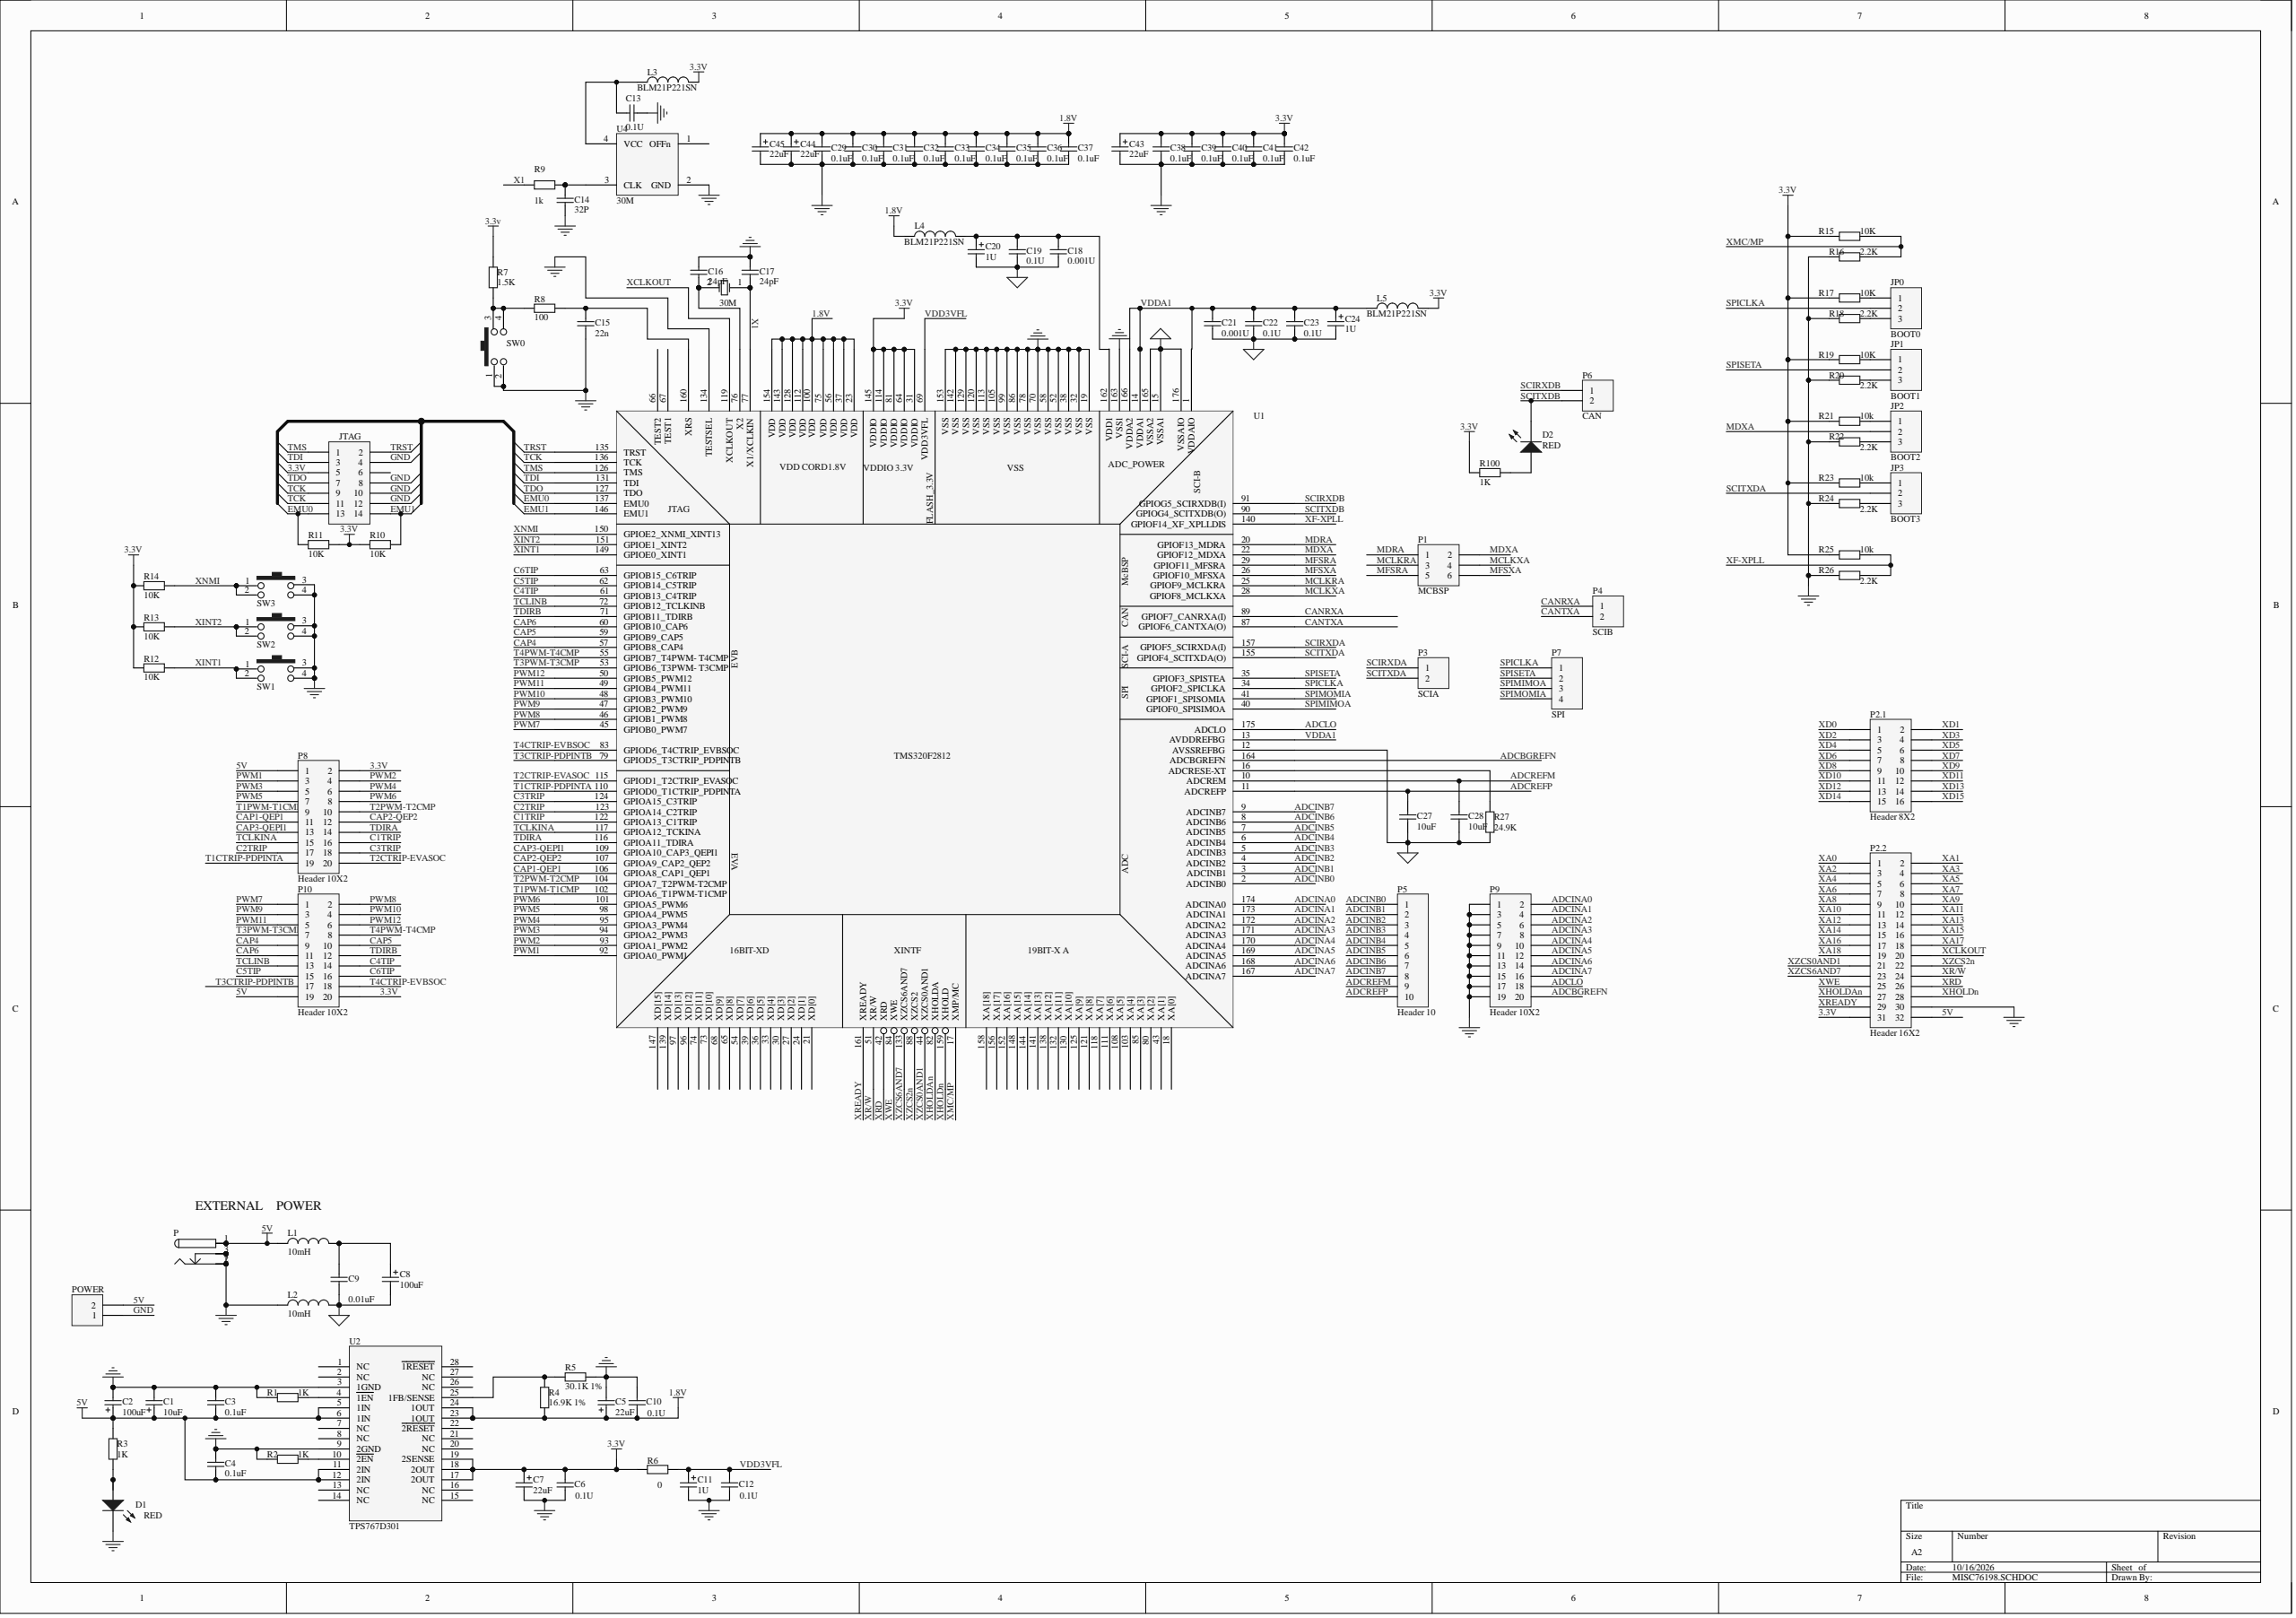Circuit board | Altium Designer | 104 parts | 123 nets
Bill of materials:
Comment,Description,Designator,Footprint,LibRef,Quantity
"XTAL","Crystal Oscillator","30M","TXAL","XTAL","1"
"Cap Pol1","Polarized Capacitor (Radial)","C1, C5, C7","C2","Cap Pol1","3"
"Cap Pol1","Polarized Capacitor (Radial)","C2, C8","C1","Cap Pol1","2"
"Cap","Capacitor","C3, C4, C6, C9, C10, C12, C13, C14, C15, C27, C28","0603","Cap","11"
"Cap Pol1","Polarized Capacitor (Radial)","C11","1210","Cap Pol1","1"
"Cap Semi","Capacitor (Semiconductor SIM Model)","C16, C17, C18, C19, C21, C22, C23","0603","Cap Semi","7"
"Cap Pol1","Polarized Capacitor (Radial)","C20, C24","0805","Cap Pol1","2"
"0.1uF","Capacitor","C29, C30, C31, C32, C33, C34, C35, C36, C37, C38, C39, C40, C41, C42","0603","Cap","14"
"Cap Pol1","Polarized Capacitor (Radial)","C43, C44, C45","1206","Cap Pol1","3"
"RED","Subminiature High Performance AlInGaP LED Lamp","D1, D2","0603","HLMA-PG00-N0011","2"
"BOOT0","Header, 3-Pin","JP0","HDR1X3","Header 3","1"
"BOOT1","Header, 3-Pin","JP1","HDR1X3","Header 3","1"
"BOOT2","Header, 3-Pin","JP2","HDR1X3","Header 3","1"
"BOOT3","Header, 3-Pin","JP3","HDR1X3","Header 3","1"
"Header 7X2","Header, 7-Pin, Dual row","JTAG","HDR2X7","Header 7X2","1"
"Inductor","Inductor","L1, L2, L3, L4, L5","0805","Inductor","5"
"PWR2.5","Low Voltage Power Supply Connector","P","KLD-0202","PWR2.5","1"
"MCBSP","Header, 3-Pin, Dual row","P1","HDR2X3","Header 3X2","1"
"Header 8X2","Header, 8-Pin, Dual row","P2.1","HDR2X8","Header 8X2","1"
"Header 16X2","Header, 16-Pin, Dual row","P2.2","HDR2X16","Header 16X2","1"
"SCIA","Header, 2-Pin","P3","HDR1X2","Header 2","1"
"SCIB","Header, 2-Pin","P4","HDR1X2","Header 2","1"
"Header 10","Header, 10-Pin","P5","HDR1X10","Header 10","1"
"CAN","Header, 2-Pin","P6","HDR1X2","Header 2","1"
"SPI","Header, 4-Pin","P7","HDR1X4","Header 4","1"
"Header 10X2","Header, 10-Pin, Dual row","P8, P9, P10","HDR2X10","Header 10X2","3"
"Header 2","Header, 2-Pin","POWER","HDR1X2","Header 2","1"
"Res2","Resistor","R1, R2, R3, R4, R5, R6, R10, R11, R12, R13, R14, R100","0603","Res2","12"
"1.5K","Resistor","R7","0603","Res2","1"
"100","Resistor","R8","0603","Res2","1"
"1k","Resistor","R9, R16","0603","Res2","2"
"10K","Resistor","R15, R17, R19, R21, R23, R25","0603","Res2","6"
"2.2K","Resistor","R18, R20, R22, R24, R26","0603","Res2","5"
"24.9K","Resistor","R27","0603","Res2","1"
"KEY4","","SW0, SW1, SW2, SW3","key","KEY4","4"
"TMS320F2812","","U1","QFP176","TMS320F2812","1"
"TPS767D301","","U2","TSOP28(0.65mm)","TPS73HD301","1"
"30M","","U4","CRYSTAL1","30M","1"
Netlist (Protel format):
[
30M
TXAL
XTAL



]
[
C1
C2
Cap Pol1



]
[
C2
C1
Cap Pol1



]
[
C3
0603
Cap



]
[
C4
0603
Cap



]
[
C5
C2
Cap Pol1



]
[
C6
0603
Cap



]
[
C7
c2
Cap Pol1



]
[
C8
C1
Cap Pol1



]
[
C9
0603
Cap



]
[
C10
0603
Cap



]
[
C11
1210
Cap Pol1



]
[
C12
0603
Cap



]
[
C13
0603
Cap



]
[
C14
0603
Cap



]
[
C15
0603
Cap



]
[
C16
0603
Cap Semi



]
[
C17
0603
Cap Semi



]
[
C18
0603
Cap Semi



]
[
C19
0603
Cap Semi



]
[
C20
0805
Cap Pol1



]
[
C21
0603
Cap Semi



]
[
C22
0603
Cap Semi



]
[
C23
0603
Cap Semi



]
[
C24
0805
Cap Pol1



]
[
C27
0603
Cap



]
[
C28
0603
Cap



]
[
C29
0603
0.1uF



]
[
C30
0603
0.1uF



]
[
C31
0603
0.1uF



]
[
C32
0603
0.1uF



]
[
C33
0603
0.1uF



]
[
C34
0603
0.1uF



]
[
C35
0603
0.1uF



]
[
C36
0603
0.1uF



]
[
C37
0603
0.1uF



]
[
C38
0603
0.1uF



]
[
C39
0603
0.1uF



]
[
C40
0603
0.1uF



]
[
C41
0603
0.1uF



]
[
C42
0603
0.1uF



]
[
C43
1206
Cap Pol1



]
[
C44
1206
Cap Pol1



]
[
C45
1206
Cap Pol1



]
[
D1
0603
RED



]
[
D2
0603
RED



]
[
JP0
HDR1X3
BOOT0



]
[
JP1
HDR1X3
BOOT1



]
[
JP2
HDR1X3
BOOT2



]
[
JP3
HDR1X3
BOOT3



]
[
JTAG
HDR2X7
Header 7X2



]
[
L1
0805
Inductor



]
[
L2
0805
Inductor



]
[
L3
0805
Inductor



]
[
L4
0805
Inductor



]
[
L5
0805
Inductor



]
[
P
KLD-0202
PWR2.5



]
[
P1
HDR2X3
MCBSP



]
[
P2.1
HDR2X8
Header 8X2



]
[
P2.2
HDR2X16
Header 16X2



]
[
P3
HDR1X2
SCIA



]
[
P4
HDR1X2
SCIB



]
[
P5
HDR1X10
Header 10



]
[
P6
HDR1X2
CAN



]
[
P7
HDR1X4
SPI



]
[
P8
HDR2X10
Header 10X2



]
[
P9
HDR2X10
Header 10X2



]
[
P10
HDR2X10
Header 10X2



]
[
POWER
HDR1X2
Header 2



]
[
R1
0603
Res2



]
[
R2
0603
Res2



]
[
R3
0603
Res2



]
[
R4
0603
Res2



]
[
R5
0603
Res2



]
[
R6
0603
Res2



]
[
R7
0603
1.5K



]
[
R8
0603
100



]
[
R9
0603
1k



]
[
R10
0603
Res2



]
[
R11
0603
Res2



]
[
R12
0603
Res2



]
[
R13
0603
Res2



]
[
R14
0603
Res2



]
[
R15
0603
10K



]
[
R16
0603
1k



]
[
R17
0603
10K



]
[
R18
0603
2.2K



]
[
R19
0603
10K



]
[
R20
0603
2.2K



]
[
R21
0603
10k



]
[
R22
0603
2.2K



]
[
R23
0603
10k



]
[
R24
0603
2.2K



]
[
R25
0603
10k



]
[
R26
0603
2.2K



]
[
R27
0603
24.9K



]
[
R100
0603
Res2



]
[
SW0
key
KEY4



]
[
SW1
key
KEY4



]
[
SW2
key
KEY4



]
[
SW3
key
KEY4



]
[
U1
QFP176
TMS320F2812



]
[
U2
TSOP28(0.65mm)
TPS767D301



]
[
U4
CRYSTAL1
30M



]
(
XZCS6AND7
P2.2-23
U1-133
)
(
XZCS2n
P2.2-22
U1-88
)
(
XZCS0AND1
P2.2-21
U1-44
)
(
XWE
P2.2-25
U1-84
)
(
XREADY
P2.2-29
U1-161
)
(
XRD
P2.2-26
U1-42
)
(
XR/W
P2.2-24
U1-51
)
(
XNMI
R14-2
SW3-1
SW3-2
U1-150
)
(
XMC/MP
R15-2
R16-2
U1-17
)
(
XINT2
R13-2
SW2-1
SW2-2
U1-151
)
(
XINT1
R12-2
SW1-1
SW1-2
U1-149
)
(
XHOLDn
P2.2-28
U1-159
)
(
XHOLDAn
P2.2-27
U1-82
)
(
XF-XPLL
R25-2
R26-2
U1-140
)
(
XCLKOUT
P2.2-20
U1-119
)
(
X1
30M-1
C17-1
R9-1
U1-77
)
(
VDDA1
C21-2
C22-2
C23-2
C24-1
L5-1
U1-1
U1-13
U1-14
U1-166
)
(
VDD3VFL
C11-1
C12-2
R6-1
U1-69
)
(
TRST
JTAG-2
U1-135
)
(
TMS
JTAG-1
U1-126
)
(
TDO
JTAG-7
U1-127
)
(
TDIRB
P10-12
U1-71
)
(
TDIRA
P8-14
U1-116
)
(
TDI
JTAG-3
U1-131
)
(
TCLKINA
P8-15
U1-117
)
(
TCLINB
P10-13
U1-72
)
(
TCK
JTAG-9
JTAG-11
U1-136
)
(
T4PWM-T4CMP
P10-8
U1-55
)
(
T4CTRIP-EVBSOC
P10-18
U1-83
)
(
T3PWM-T3CMP
P10-7
U1-53
)
(
T3CTRIP-PDPINTB
P10-17
U1-79
)
(
T2PWM-T2CMP
P8-10
U1-104
)
(
T2CTRIP-EVASOC
P8-20
U1-115
)
(
T1PWM-T1CMP
P8-9
U1-102
)
(
T1CTRIP-PDPINTA
P8-19
U1-110
)
(
SPISETA
JP1-2
P7-2
U1-35
)
(
SPIMOMIA
P7-4
U1-41
)
(
SPIMIMOA
P7-3
U1-40
)
(
SPICLKA
JP0-2
P7-1
U1-34
)
(
SCITXDB
D2-2
P6-2
U1-90
)
(
SCITXDA
JP3-2
P3-2
U1-155
)
(
SCIRXDB
P6-1
U1-91
)
(
SCIRXDA
P3-1
U1-157
)
(
PWM12
P10-6
U1-50
)
(
PWM11
P10-5
U1-49
)
(
PWM10
P10-4
U1-48
)
(
PWM9
P10-3
U1-47
)
(
PWM8
P10-2
U1-46
)
(
PWM7
P10-1
U1-45
)
(
PWM6
P8-8
U1-101
)
(
PWM5
P8-7
U1-98
)
(
PWM4
P8-6
U1-95
)
(
PWM3
P8-5
U1-94
)
(
PWM2
P8-4
U1-93
)
(
PWM1
P8-3
U1-92
)
(
NetR27_1
R27-1
U1-16
)
(
NetR7_1
R7-1
R8-1
SW0-3
SW0-4
)
(
NetR4_2
R4-2
R5-1
U2-25
)
(
NetR2_2
R2-2
U2-10
)
(
NetR1_2
R1-2
U2-4
)
(
NetJP3_3
JP3-3
R24-2
)
(
NetJP3_1
JP3-1
R23-2
)
(
NetJP2_3
JP2-3
R22-2
)
(
NetJP2_1
JP2-1
R21-2
)
(
NetJP1_3
JP1-3
R20-2
)
(
NetJP1_1
JP1-1
R19-2
)
(
NetJP0_3
JP0-3
R18-2
)
(
NetJP0_1
JP0-1
R17-2
)
(
NetD2_1
D2-1
R100-2
)
(
NetD1_1
D1-1
R3-1
)
(
NetC18_2
C18-2
C19-2
C20-1
L4-2
U1-162
)
(
NetC15_2
C15-2
R8-2
U1-160
)
(
NetC14_2
C14-2
R9-2
U4-3
)
(
NetC13_2
C13-2
L3-1
U4-4
)
(
NetC8_1
C8-1
C9-2
L1-2
)
(
Net30M_2
30M-2
C16-2
U1-76
)
(
MFSXA
P1-6
U1-26
)
(
MFSRA
P1-5
U1-29
)
(
MDXA
JP2-2
P1-2
U1-22
)
(
MDRA
P1-1
U1-20
)
(
MCLKXA
P1-4
U1-28
)
(
MCLKRA
P1-3
U1-25
)
(
GND
C1-2
C2-2
C3-2
C4-1
C5-2
C6-1
C7-2
C10-2
C11-2
C12-1
C13-1
C14-1
C15-1
C16-1
C17-2
C29-2
C30-1
C31-1
C32-1
C33-1
C34-1
C35-1
C36-1
C37-1
C38-1
C39-1
C40-1
C41-2
C42-1
C43-2
C44-2
C45-2
D1-2
JTAG-4
JTAG-8
JTAG-10
JTAG-12
L2-1
P-2
P-2A
P-2B
P-3
P-3A
P-3B
P2.2-30
P9-1
P9-3
P9-5
P9-7
P9-9
P9-11
P9-13
P9-15
P9-17
P9-19
POWER-1
R1-1
R2-1
R5-2
R16-1
R18-1
R20-1
R22-1
R24-1
R26-1
SW0-1
SW0-2
SW1-3
SW1-4
SW2-3
SW2-4
SW3-3
SW3-4
U1-19
U1-32
U1-38
U1-52
U1-58
U1-70
U1-78
U1-86
U1-99
U1-105
U1-113
U1-120
U1-129
U1-134
U1-142
U1-153
U1-163
U2-3
U2-9
U4-2
)
(
EMU1
JTAG-14
R10-1
U1-146
)
(
EMU0
JTAG-13
R11-1
U1-137
)
(
CAP6
P10-11
U1-60
)
(
CAP5
P10-10
U1-59
)
(
CAP4
P10-9
U1-57
)
(
CAP3-QEPI1
P8-13
U1-109
)
(
CAP2-QEP2
P8-12
U1-107
)
(
CAP1-QEP1
P8-11
U1-106
)
(
CANTXA
P4-2
U1-87
)
(
CANRXA
P4-1
U1-89
)
(
C6TIP
P10-16
U1-63
)
(
C5TIP
P10-15
U1-62
)
(
C4TIP
P10-14
U1-61
)
(
C3TRIP
P8-18
U1-124
)
(
C2TRIP
P8-17
U1-123
)
(
C1TRIP
P8-16
U1-122
)
(
AGND
C8-2
C9-1
C18-1
C19-1
C20-2
C21-1
C22-1
C23-1
C24-2
C27-2
C28-2
L2-2
R27-2
U1-12
U1-15
U1-165
U1-176
)
(
ADCREFP
C27-1
P5-10
U1-11
)
(
ADCREFM
C28-1
P5-9
U1-10
)
(
ADCLO
P9-18
U1-175
)
(
ADCINB7
P5-8
U1-9
)
(
ADCINB6
P5-7
U1-8
)
(
ADCINB5
P5-6
U1-7
)
(
ADCINB4
P5-5
U1-6
)
(
ADCINB3
P5-4
U1-5
)
(
ADCINB2
P5-3
U1-4
)
(
ADCINB1
P5-2
U1-3
)
(
ADCINB0
P5-1
U1-2
)
(
ADCINA7
P9-16
U1-167
)
(
ADCINA6
P9-14
U1-168
)
(
ADCINA5
P9-12
U1-169
)
(
ADCINA4
P9-10
U1-170
)
(
ADCINA3
P9-8
U1-171
)
(
ADCINA2
P9-6
U1-172
)
(
ADCINA1
P9-4
U1-173
)
(
ADCINA0
P9-2
U1-174
)
(
ADCBGREFN
P9-20
U1-164
)
(
5V
C1-1
C2-1
C3-1
C4-2
L1-1
P-1
P-1A
P-1B
P2.2-32
P8-1
P10-19
POWER-2
R3-2
U2-5
U2-6
U2-11
U2-12
)
(
3.3V
C6-2
C7-1
C38-2
C39-2
C40-2
C41-1
C42-2
C43-1
JTAG-5
L3-2
L5-2
P2.2-31
P8-2
P10-20
R6-2
R7-2
R10-2
R11-2
R12-1
R13-1
R14-1
R15-1
R17-1
R19-1
R21-1
R23-1
R25-1
R100-1
U1-31
U1-64
U1-81
U1-114
U1-145
U2-17
U2-18
U2-19
)
(
1.8V
C5-1
C10-1
C29-1
C30-2
C31-2
C32-2
C33-2
C34-2
C35-2
C36-2
C37-2
C44-1
C45-1
L4-1
R4-1
U1-23
U1-37
U1-56
U1-75
U1-100
U1-112
U1-128
U1-143
U1-154
U2-23
U2-24
)